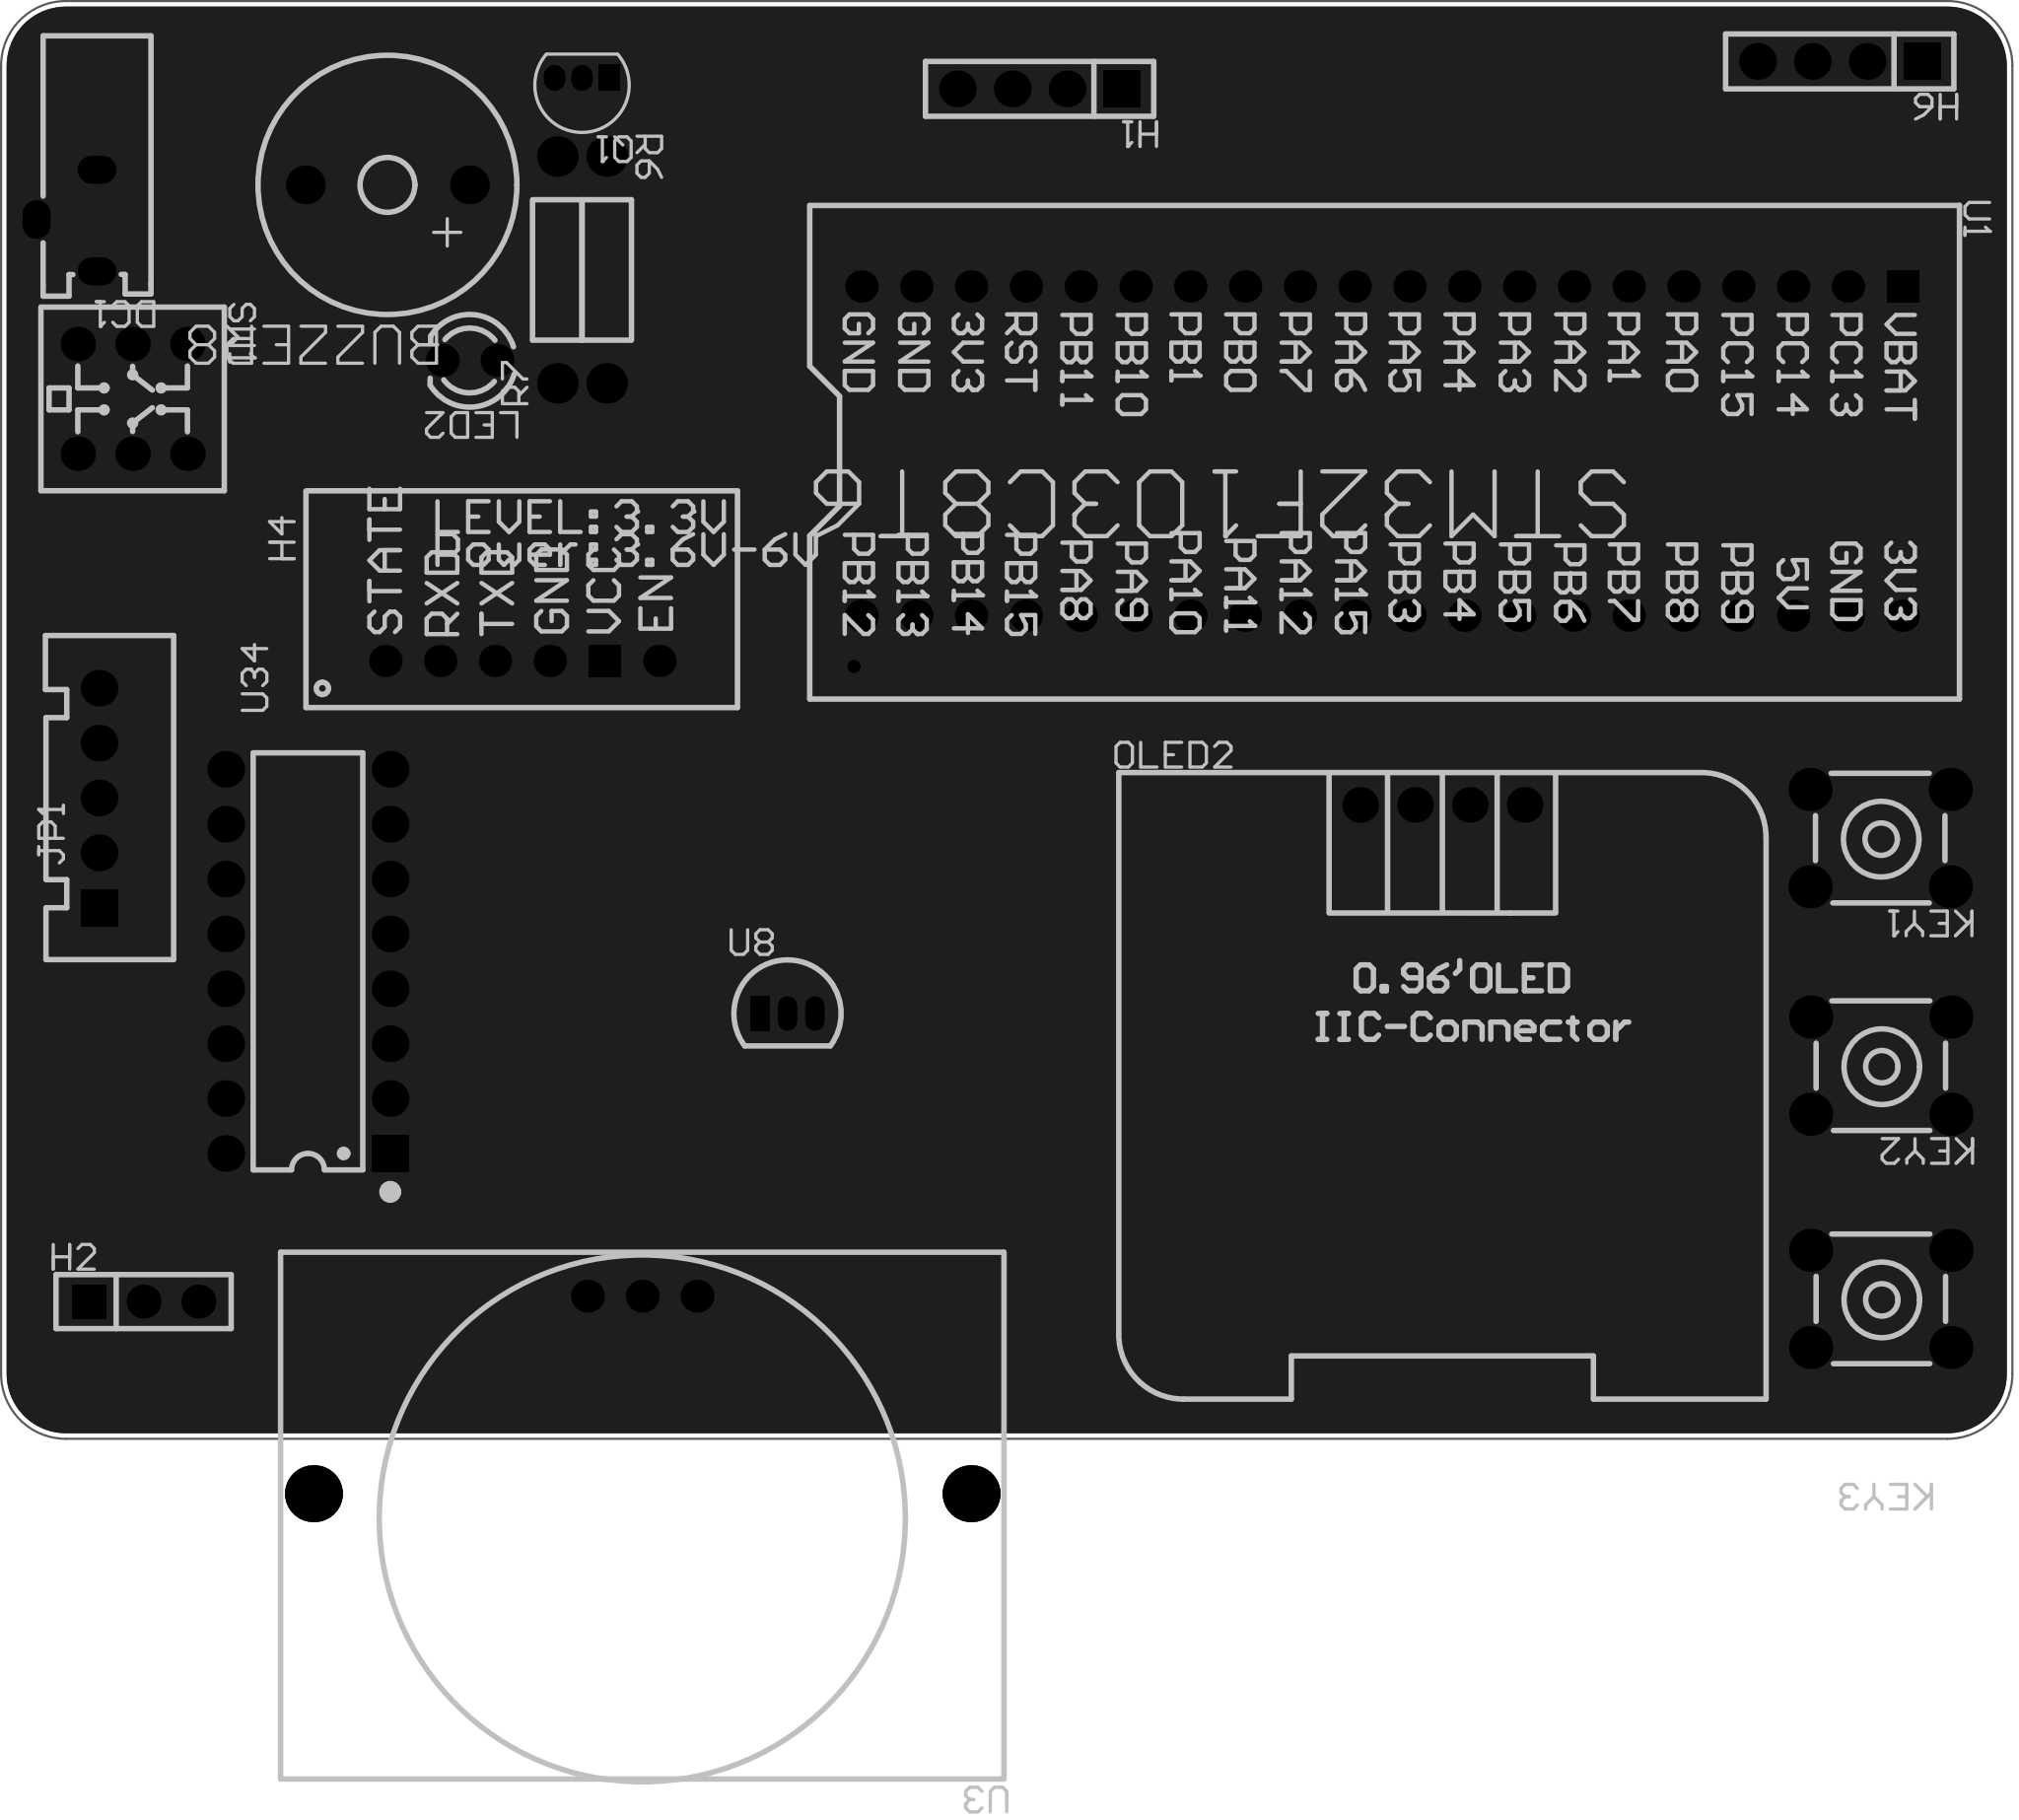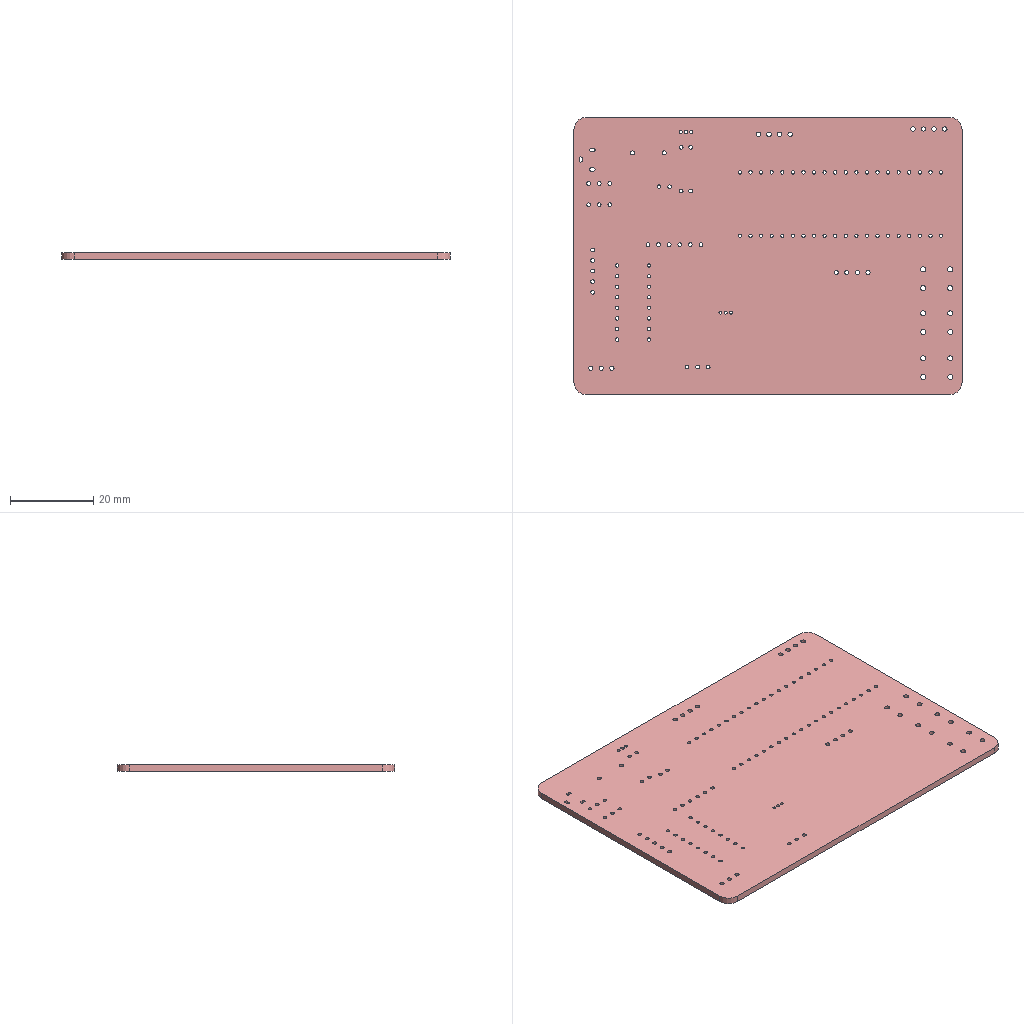Circuit board layout | Altium Designer | box 93.2 x 66.5 x 1.6 mm
Layer stack:
# Altium Designer layer stack of  (unit mm; dielectric type: 0 none, 1 core, 2 prepreg, 3 surface material)
index,name,kind,layer,copper_thickness_mm,dielectric_type,dielectric_thickness_mm,dielectric_material,dielectric_constant
0,Top Paste Mask Layer,other,,,,,,
1,Top Silkscreen Layer,other,,,,,,
2,Top Solder Mask Layer,dielectric,,,3,0.01,,3.3
3,Top Layer,copper,Top Layer,0.035,,,,
4,Dielectric1,dielectric,,,3,1.51,FR4,4.5
5,Bottom Layer,copper,Bottom Layer,0.035,,,,
6,Bottom Solder Mask Layer,dielectric,,,3,0.01,,3.3
7,Bottom Silkscreen Layer,other,,,,,,
8,Bottom Paste Mask Layer,other,,,,,,
# drill layer pairs: low layer,high layer
drill_pair,Top Layer,Bottom Layer
Part placement:
Designator,Comment,Layer,Footprint,Center-X(mm),Center-Y(mm),Rotation
DC1,DC002-1.3,TopLayer,DC-IN-TH_DC002-1.3,95.885,157.912,180
KEY1,Tact switch 6*6*8,TopLayer,KEY-TH_4P-L6.0-W6.0-P4.50-LS7.5,179.93,129.328,180
KEY2,Tact switch 6*6*8,TopLayer,KEY-TH_4P-L6.0-W6.0-P4.50-LS7.5,179.959,118.796,180
KEY3,Tact switch 6*6*8,TopLayer,KEY-TH_4P-L6.0-W6.0-P4.50-LS7.5,179.959,108.001,180
H6,2.54-1*4P female,TopLayer,HDR-TH_4P-P2.54-V-F,178.054,165.278,180
SW1,,TopLayer,自锁开关8.5*8.5,98.933,149.657,270
OLED2,0.96OLED_4P_MODULE_JX,TopLayer,0.96OLED_4P,159.639,130.861,0
R7,,TopLayer,RES-TH_BD2.3-L6.5-P10.50-D0.5,118.618,155.626,90
R6,,TopLayer,RES-TH_BD2.3-L6.5-P10.50-D0.5,120.904,155.626,270
Q1,S8550,TopLayer,TO-92-3_L4.5-W3.5-P1.27-L,119.761,164.516,180
LED2,,TopLayer,LED_TH-3mm,114.554,151.435,180
BUZZER8,buzzer-12X9,TopLayer,BUZ-TH_BD12.0-P7.60-D0.6-FD,110.744,159.563,180
H1,2.54-1*4P female,TopLayer,HDR-TH_4P-P2.54-V-F,140.97,164.008,180
DRIVER1,Darlington driver IC,TopLayer,DIP-16,107.061,123.622,180
JP1,HDR-1X5,TopLayer,XH2.54-LI-5P,97.38,131.184,90
U3,HC-SR501 PIR sensor module,TopLayer,HC-SR501,122.555,103.556,180
U1,STM32F103C8T6-Bluepill,TopLayer,STM32F103C8T6-BLUEPILL,156.845,147.244,270
U34,,TopLayer,蓝牙level,117,137.529,90
U8,DS18B20,TopLayer,TO-92-3_L4.9-W3.7-P1.27-L,129.286,121.209,0
H2,,TopLayer,HDR-TH_3P-P2.54-V-F,99.441,107.874,0
Pad and via stacks:
# Altium Designer via and pad stacks of  (unit mm). Each distinct definition once, with the count of objects using it.
# via: kind,start_layer,end_layer,hole_mm,diameter_mm,mode(0 simple;1 top-mid-bottom;2 full stack),diameter_per_layer,count,example_net
# pad: kind,layer,hole_mm,hole_type(0 round;1 square;2 slot),plating,top_size,top_shape(1 round;2 rect;3 octagon;9 rounded rect),mid_size,bottom_size,mode,footprint,size_per_layer,count,example
pad,Multi-Layer,0.8,2,plated,1.3x1.8,1,1.3x1.8,1.3x1.8,0,DC-IN-TH_DC002-1.3,,3,DC1.1
pad,Multi-Layer,1.2,0,plated,2x2,1,2x2,2x2,0,KEY-TH_4P-L6.0-W6.0-P4.50-LS7.5,,12,KEY1.1
pad,Multi-Layer,1.1,0,plated,1.7x1.7,2,1.7x1.7,1.7x1.7,0,HDR-TH_4P-P2.54-V-F,,2,H6.1
pad,Multi-Layer,1.1,0,plated,1.7x1.7,1,1.7x1.7,1.7x1.7,0,HDR-TH_4P-P2.54-V-F,,6,H6.2
pad,Multi-Layer,0.9,0,plated,1.6x1.6,1,1.6x1.6,1.6x1.6,0,\u00D7\u00D4\u00CB\u00F8\u00BF\u00AA\u00B9\u00D88.5*8.5,,6,SW1.1
pad,Multi-Layer,1,0,plated,1.65x1.65,1,1.65x1.65,1.65x1.65,0,0.96OLED_4P,,4,OLED2.4
pad,Multi-Layer,0.8992,0,plated,1.88x1.88,1,1.88x1.88,1.88x1.88,0,RES-TH_BD2.3-L6.5-P10.50-D0.5,,4,R7.1
pad,Multi-Layer,0.7,2,plated,1x1.2,2,1x1.2,1x1.2,0,TO-92-3_L4.5-W3.5-P1.27-L,,1,Q1.1
pad,Multi-Layer,0.7,2,plated,1x1.2,1,1x1.2,1x1.2,0,TO-92-3_L4.5-W3.5-P1.27-L,,2,Q1.2
pad,Multi-Layer,0.9144,0,plated,1.524x1.524,1,1.524x1.524,1.524x1.524,0,LED_TH-3mm,,2,LED2.1
pad,Multi-Layer,1.001,0,plated,1.801x1.801,1,1.801x1.801,1.801x1.801,0,BUZ-TH_BD12.0-P7.60-D0.6-FD,,2,BUZZER8.1
pad,Multi-Layer,0.8,0,plated,1.7x1.7,1,1.7x1.7,1.7x1.7,0,DIP-16,,15,DRIVER1.16
pad,Multi-Layer,0.8,0,plated,1.7x1.7,2,1.7x1.7,1.7x1.7,0,DIP-16,,1,DRIVER1.1
pad,Multi-Layer,0.9,0,plated,1.7x1.7,1,1.7x1.7,1.7x1.7,0,XH2.54-LI-5P,,4,JP1.5
pad,Multi-Layer,0.9,0,plated,1.7x1.7,2,1.7x1.7,1.7x1.7,0,XH2.54-LI-5P,,1,JP1.1
pad,Multi-Layer,2.032,0,plated,2.642x2.642,1,2.642x2.642,2.642x2.642,0,HC-SR501,,2,U3.
pad,Multi-Layer,0.914,0,plated,1.524x1.524,1,1.524x1.524,1.524x1.524,0,HC-SR501,,3,U3.1
pad,Multi-Layer,0.8,0,plated,1.5x1.5,1,1.5x1.5,1.5x1.5,0,STM32F103C8T6-BLUEPILL,,39,U1.40
pad,Multi-Layer,0.8,0,plated,1.5x1.5,2,1.5x1.5,1.5x1.5,0,STM32F103C8T6-BLUEPILL,,1,U1.1
pad,Multi-Layer,0.9,2,plated,1.5x1.5,2,1.5x1.5,1.5x1.5,0,\u00C0\u00B6\u00D1\u00C0level,,1,U34.5
pad,Multi-Layer,0.9,2,plated,1.5x1.5,1,1.5x1.5,1.5x1.5,0,\u00C0\u00B6\u00D1\u00C0level,,5,U34.6
pad,Multi-Layer,0.7,0,plated,0.9x1.6,1,0.9x1.6,0.9x1.6,0,TO-92-3_L4.9-W3.7-P1.27-L,,2,U8.3
pad,Multi-Layer,0.7,0,plated,0.9x1.6,2,0.9x1.6,0.9x1.6,0,TO-92-3_L4.9-W3.7-P1.27-L,,1,U8.1
pad,Multi-Layer,1.02,0,plated,1.575x1.575,1,1.575x1.575,1.575x1.575,0,HDR-TH_3P-P2.54-V-F,,2,H2.3
pad,Multi-Layer,1.02,0,plated,1.575x1.575,2,1.575x1.575,1.575x1.575,0,HDR-TH_3P-P2.54-V-F,,1,H2.1
via,Top Layer,Bottom Layer,0.3048,0.61,0,,1,PB14
Copper pours:
name,layer,net,type(0 solid;1 hatched;2 none)
Top Layer-GND,Top Layer,GND,0
Bottom Layer-GND,Bottom Layer,GND,0
Design rules, without the lines most boards share:
# Altium Designer design rules of  (exported by Altium Designer, unit mm)
# columns: name | kind | enabled | priority | scope1 | scope2 | descriptor | typed fields (field=value)
copperThickness1oz_2 | 2 | enabled | 2 | All | All | Width Constraint (Min=5mil) (Max=100mil) (Preferred=19.7mil) (All) |